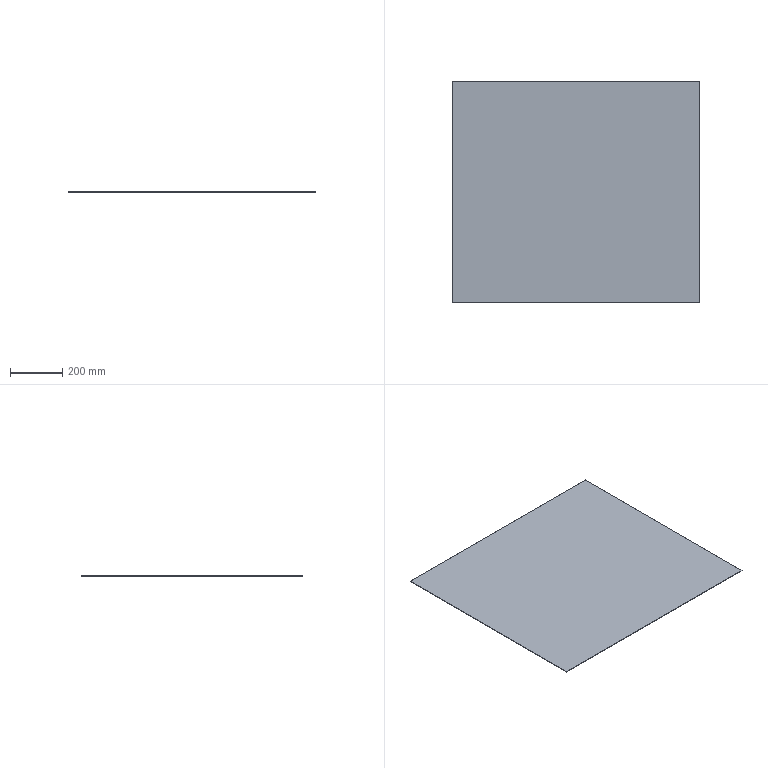Part | STEP file | Upper frame acrylic cover plate | 1 solid | 6 faces | box 948.003 x 848 x 2 mm | volume 1607813 mm3 | plane 6
STEP:
#1=CARTESIAN_POINT('',(0.,0.,0.));
#2=VERTEX_POINT('',#1);
#3=CARTESIAN_POINT('',(0.,-848.,0.));
#4=VERTEX_POINT('',#3);
#5=CARTESIAN_POINT('',(0.,0.,0.));
#6=DIRECTION('',(0.,-1.,0.));
#7=VECTOR('',#6,1000.);
#8=LINE('',#5,#7);
#9=EDGE_CURVE('',#2,#4,#8,.T.);
#10=ORIENTED_EDGE('',*,*,#9,.T.);
#11=CARTESIAN_POINT('',(0.,-848.,2.));
#12=VERTEX_POINT('',#11);
#13=CARTESIAN_POINT('',(0.,-848.,2.));
#14=DIRECTION('',(0.,0.,-1.));
#15=VECTOR('',#14,1000.);
#16=LINE('',#13,#15);
#17=EDGE_CURVE('',#12,#4,#16,.T.);
#18=ORIENTED_EDGE('',*,*,#17,.F.);
#19=CARTESIAN_POINT('',(0.,0.,2.));
#20=VERTEX_POINT('',#19);
#21=CARTESIAN_POINT('',(0.,0.,2.));
#22=DIRECTION('',(0.,-1.,0.));
#23=VECTOR('',#22,1000.);
#24=LINE('',#21,#23);
#25=EDGE_CURVE('',#20,#12,#24,.T.);
#26=ORIENTED_EDGE('',*,*,#25,.F.);
#27=CARTESIAN_POINT('',(0.,0.,2.));
#28=DIRECTION('',(0.,0.,-1.));
#29=VECTOR('',#28,1000.);
#30=LINE('',#27,#29);
#31=EDGE_CURVE('',#20,#2,#30,.T.);
#32=ORIENTED_EDGE('',*,*,#31,.T.);
#33=EDGE_LOOP('',(#10,#18,#26,#32));
#34=FACE_OUTER_BOUND('',#33,.T.);
#35=CARTESIAN_POINT('',(0.,0.,2.));
#36=DIRECTION('',(1.,0.,0.));
#37=DIRECTION('',(0.,1.,0.));
#38=AXIS2_PLACEMENT_3D('',#35,#36,#37);
#39=PLANE('',#38);
#40=ADVANCED_FACE('',(#34),#39,.F.);
#41=CARTESIAN_POINT('',(948.003,-848.,0.));
#42=VERTEX_POINT('',#41);
#43=CARTESIAN_POINT('',(0.,-848.,0.));
#44=DIRECTION('',(1.,0.,0.));
#45=VECTOR('',#44,1000.);
#46=LINE('',#43,#45);
#47=EDGE_CURVE('',#4,#42,#46,.T.);
#48=ORIENTED_EDGE('',*,*,#47,.T.);
#49=CARTESIAN_POINT('',(948.003,-848.,2.));
#50=VERTEX_POINT('',#49);
#51=CARTESIAN_POINT('',(948.003,-848.,2.));
#52=DIRECTION('',(0.,0.,-1.));
#53=VECTOR('',#52,1000.);
#54=LINE('',#51,#53);
#55=EDGE_CURVE('',#50,#42,#54,.T.);
#56=ORIENTED_EDGE('',*,*,#55,.F.);
#57=CARTESIAN_POINT('',(0.,-848.,2.));
#58=DIRECTION('',(1.,0.,0.));
#59=VECTOR('',#58,1000.);
#60=LINE('',#57,#59);
#61=EDGE_CURVE('',#12,#50,#60,.T.);
#62=ORIENTED_EDGE('',*,*,#61,.F.);
#63=ORIENTED_EDGE('',*,*,#17,.T.);
#64=EDGE_LOOP('',(#48,#56,#62,#63));
#65=FACE_OUTER_BOUND('',#64,.T.);
#66=CARTESIAN_POINT('',(0.,-848.,2.));
#67=DIRECTION('',(0.,1.,0.));
#68=DIRECTION('',(0.,0.,1.));
#69=AXIS2_PLACEMENT_3D('',#66,#67,#68);
#70=PLANE('',#69);
#71=ADVANCED_FACE('',(#65),#70,.F.);
#72=CARTESIAN_POINT('',(948.003,0.,0.));
#73=VERTEX_POINT('',#72);
#74=CARTESIAN_POINT('',(948.003,0.,0.));
#75=DIRECTION('',(0.,1.,0.));
#76=VECTOR('',#75,1000.);
#77=LINE('',#74,#76);
#78=EDGE_CURVE('',#42,#73,#77,.T.);
#79=ORIENTED_EDGE('',*,*,#78,.T.);
#80=CARTESIAN_POINT('',(948.003,0.,2.));
#81=VERTEX_POINT('',#80);
#82=CARTESIAN_POINT('',(948.003,0.,2.));
#83=DIRECTION('',(0.,0.,-1.));
#84=VECTOR('',#83,1000.);
#85=LINE('',#82,#84);
#86=EDGE_CURVE('',#81,#73,#85,.T.);
#87=ORIENTED_EDGE('',*,*,#86,.F.);
#88=CARTESIAN_POINT('',(948.003,0.,2.));
#89=DIRECTION('',(0.,1.,0.));
#90=VECTOR('',#89,1000.);
#91=LINE('',#88,#90);
#92=EDGE_CURVE('',#50,#81,#91,.T.);
#93=ORIENTED_EDGE('',*,*,#92,.F.);
#94=ORIENTED_EDGE('',*,*,#55,.T.);
#95=EDGE_LOOP('',(#79,#87,#93,#94));
#96=FACE_OUTER_BOUND('',#95,.T.);
#97=CARTESIAN_POINT('',(948.003,0.,2.));
#98=DIRECTION('',(-1.,0.,0.));
#99=DIRECTION('',(0.,0.,1.));
#100=AXIS2_PLACEMENT_3D('',#97,#98,#99);
#101=PLANE('',#100);
#102=ADVANCED_FACE('',(#96),#101,.F.);
#103=CARTESIAN_POINT('',(0.,0.,0.));
#104=DIRECTION('',(-1.,0.,0.));
#105=VECTOR('',#104,1000.);
#106=LINE('',#103,#105);
#107=EDGE_CURVE('',#73,#2,#106,.T.);
#108=ORIENTED_EDGE('',*,*,#107,.T.);
#109=ORIENTED_EDGE('',*,*,#31,.F.);
#110=CARTESIAN_POINT('',(0.,0.,2.));
#111=DIRECTION('',(-1.,0.,0.));
#112=VECTOR('',#111,1000.);
#113=LINE('',#110,#112);
#114=EDGE_CURVE('',#81,#20,#113,.T.);
#115=ORIENTED_EDGE('',*,*,#114,.F.);
#116=ORIENTED_EDGE('',*,*,#86,.T.);
#117=EDGE_LOOP('',(#108,#109,#115,#116));
#118=FACE_OUTER_BOUND('',#117,.T.);
#119=CARTESIAN_POINT('',(0.,0.,2.));
#120=DIRECTION('',(0.,-1.,0.));
#121=DIRECTION('',(0.,0.,-1.));
#122=AXIS2_PLACEMENT_3D('',#119,#120,#121);
#123=PLANE('',#122);
#124=ADVANCED_FACE('',(#118),#123,.F.);
#125=ORIENTED_EDGE('',*,*,#25,.T.);
#126=ORIENTED_EDGE('',*,*,#61,.T.);
#127=ORIENTED_EDGE('',*,*,#92,.T.);
#128=ORIENTED_EDGE('',*,*,#114,.T.);
#129=EDGE_LOOP('',(#125,#126,#127,#128));
#130=FACE_OUTER_BOUND('',#129,.T.);
#131=CARTESIAN_POINT('',(0.,0.,2.));
#132=DIRECTION('',(0.,0.,1.));
#133=DIRECTION('',(1.,0.,0.));
#134=AXIS2_PLACEMENT_3D('',#131,#132,#133);
#135=PLANE('',#134);
#136=ADVANCED_FACE('',(#130),#135,.T.);
#137=ORIENTED_EDGE('',*,*,#9,.F.);
#138=ORIENTED_EDGE('',*,*,#107,.F.);
#139=ORIENTED_EDGE('',*,*,#78,.F.);
#140=ORIENTED_EDGE('',*,*,#47,.F.);
#141=EDGE_LOOP('',(#137,#138,#139,#140));
#142=FACE_OUTER_BOUND('',#141,.T.);
#143=CARTESIAN_POINT('',(0.,0.,0.));
#144=DIRECTION('',(0.,0.,1.));
#145=DIRECTION('',(1.,0.,0.));
#146=AXIS2_PLACEMENT_3D('',#143,#144,#145);
#147=PLANE('',#146);
#148=ADVANCED_FACE('',(#142),#147,.F.);
#149=CLOSED_SHELL('',(#40,#71,#102,#124,#136,#148));
#150=MANIFOLD_SOLID_BREP('',#149);
#151=CARTESIAN_POINT('',(0.,0.,0.));
#152=DIRECTION('',(0.,0.,1.));
#153=DIRECTION('',(1.,0.,0.));
#154=AXIS2_PLACEMENT_3D('',#151,#152,#153);
#155=(LENGTH_UNIT()NAMED_UNIT(*)SI_UNIT(.MILLI.,.METRE.));
#156=UNCERTAINTY_MEASURE_WITH_UNIT(LENGTH_MEASURE(0.00001),#155,'','');
#157=(NAMED_UNIT(*)PLANE_ANGLE_UNIT()SI_UNIT($,.RADIAN.));
#158=(NAMED_UNIT(*)SI_UNIT($,.STERADIAN.)SOLID_ANGLE_UNIT());
#159=(GEOMETRIC_REPRESENTATION_CONTEXT(3)GLOBAL_UNCERTAINTY_ASSIGNED_CONTEXT((#156))GLOBAL_UNIT_ASSIGNED_CONTEXT((#155,#157,#158))REPRESENTATION_CONTEXT('',''));
#160=ADVANCED_BREP_SHAPE_REPRESENTATION('',(#150,#154),#159);